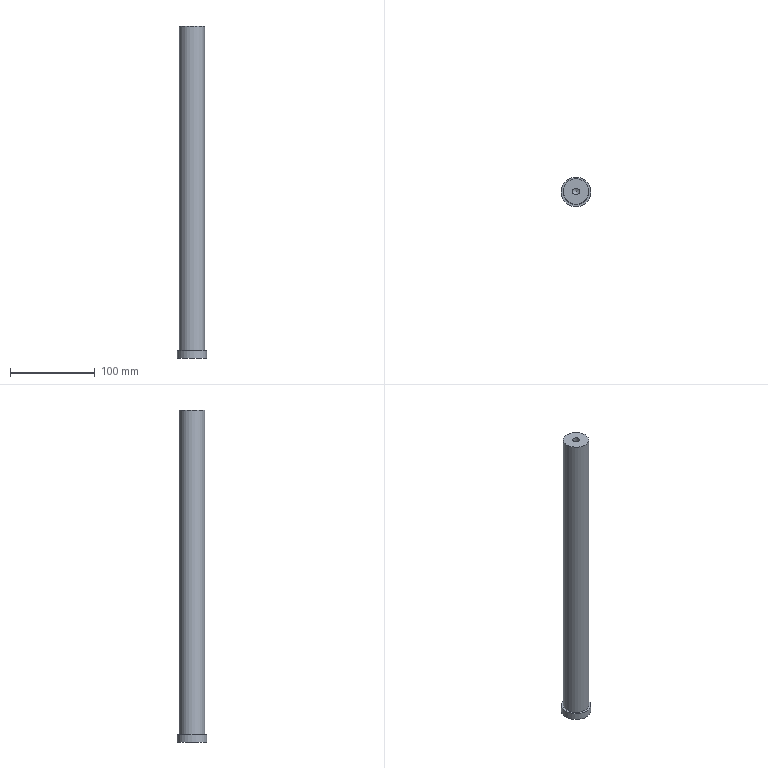Part | STEP file | solid 24 | 1 solid | 7 faces | box 35 x 35 x 391 mm | volume 277592 mm3 | cylinder 3 | plane 3 | cone 1 | commonest cylinder face diameters 8 x1 30 x1 35 x1